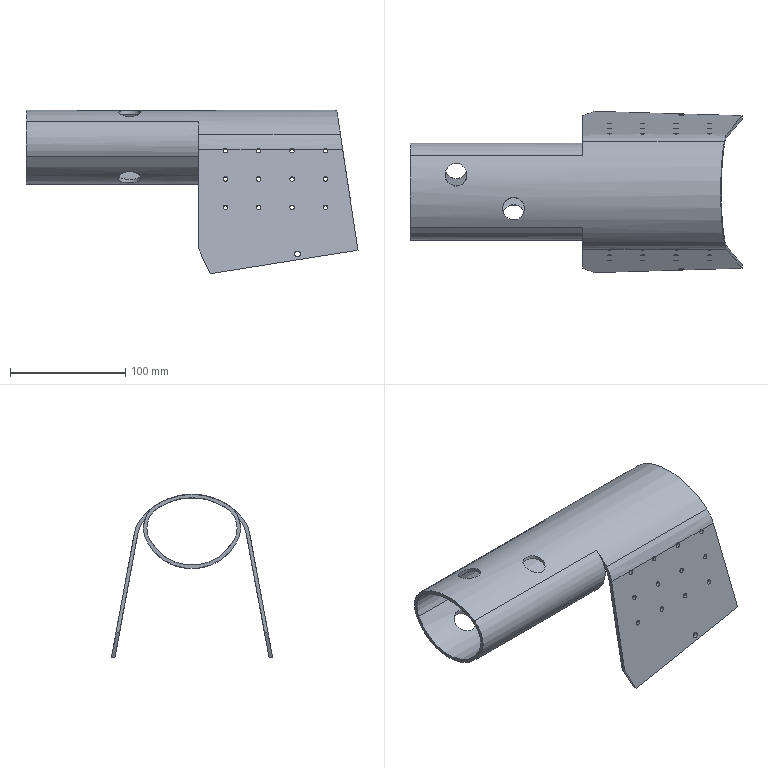Part | STEP file | 1-57.1 | 1 solid | 55 faces | box 288.5 x 140.126 x 141.936 mm | volume 221240 mm3 | cylinder 42 | plane 13 | commonest cylinder face diameters 4 x24 19 x4 5 x2 42 x2 48 x2 51 x2